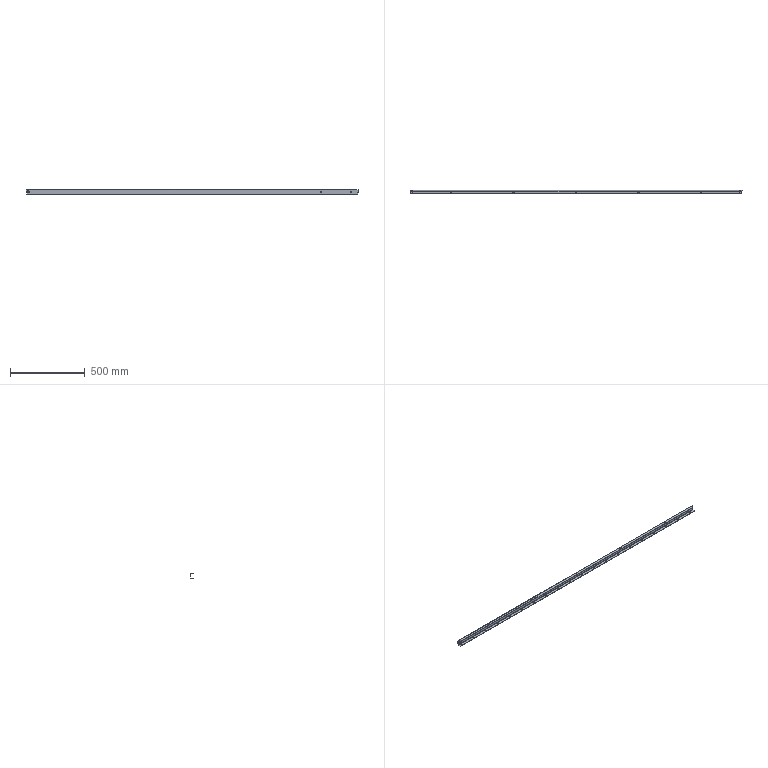Part | NX | features solid 2 | 1 solid | 78 faces | box 2215 x 20 x 38 mm | volume 311827 mm3 | cylinder 60 | plane 18 | commonest cylinder face diameters 7 x40 9.2 x14 4 x2 8 x2 15 x2